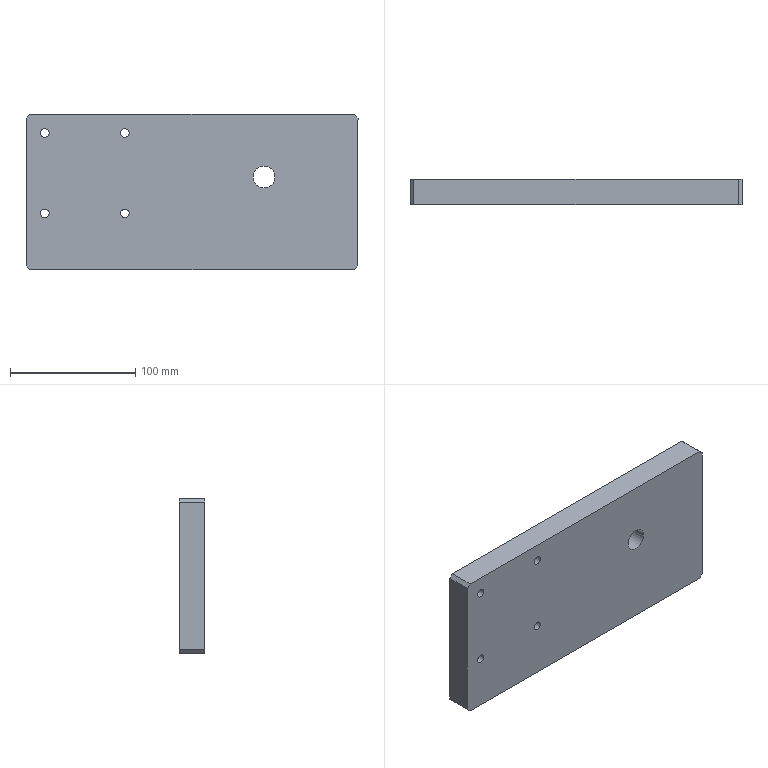Part | NX | 1 solid | 15 faces | box 265 x 20 x 124 mm | volume 649124 mm3 | plane 10 | cylinder 5 | commonest cylinder face diameters 6.8 x4 17.5 x1
STEP:
#1=CARTESIAN_POINT('',(-349.504,-20.,-263.815));
#2=VERTEX_POINT('',#1);
#3=CARTESIAN_POINT('',(-608.504,-20.,-263.815));
#4=VERTEX_POINT('',#3);
#5=CARTESIAN_POINT('',(-346.504,-20.,-263.815));
#6=DIRECTION('',(-1.,0.,0.));
#7=VECTOR('',#6,1000.);
#8=LINE('',#5,#7);
#9=EDGE_CURVE('',#2,#4,#8,.T.);
#10=ORIENTED_EDGE('',*,*,#9,.F.);
#11=CARTESIAN_POINT('',(-349.504,0.,-263.815));
#12=VERTEX_POINT('',#11);
#13=CARTESIAN_POINT('',(-349.504,-20.,-263.815));
#14=DIRECTION('',(0.,1.,0.));
#15=VECTOR('',#14,1000.);
#16=LINE('',#13,#15);
#17=EDGE_CURVE('',#2,#12,#16,.T.);
#18=ORIENTED_EDGE('',*,*,#17,.T.);
#19=CARTESIAN_POINT('',(-608.504,0.,-263.815));
#20=VERTEX_POINT('',#19);
#21=CARTESIAN_POINT('',(-346.504,0.,-263.815));
#22=DIRECTION('',(-1.,0.,0.));
#23=VECTOR('',#22,1000.);
#24=LINE('',#21,#23);
#25=EDGE_CURVE('',#12,#20,#24,.T.);
#26=ORIENTED_EDGE('',*,*,#25,.T.);
#27=CARTESIAN_POINT('',(-608.504,-20.,-263.815));
#28=DIRECTION('',(0.,-1.,0.));
#29=VECTOR('',#28,1000.);
#30=LINE('',#27,#29);
#31=EDGE_CURVE('',#20,#4,#30,.T.);
#32=ORIENTED_EDGE('',*,*,#31,.T.);
#33=EDGE_LOOP('',(#10,#18,#26,#32));
#34=FACE_BOUND('',#33,.T.);
#35=CARTESIAN_POINT('',(-346.504,-20.,-263.815));
#36=DIRECTION('',(0.,0.,-1.));
#37=DIRECTION('',(-1.,0.,0.));
#38=AXIS2_PLACEMENT_3D('',#35,#36,#37);
#39=PLANE('',#38);
#40=ADVANCED_FACE('',(#34),#39,.F.);
#41=CARTESIAN_POINT('',(-611.504,0.,-266.815));
#42=VERTEX_POINT('',#41);
#43=CARTESIAN_POINT('',(-611.504,0.,-384.815));
#44=VERTEX_POINT('',#43);
#45=CARTESIAN_POINT('',(-611.504,0.,-263.815));
#46=DIRECTION('',(0.,0.,-1.));
#47=VECTOR('',#46,1000.);
#48=LINE('',#45,#47);
#49=EDGE_CURVE('',#42,#44,#48,.T.);
#50=ORIENTED_EDGE('',*,*,#49,.T.);
#51=CARTESIAN_POINT('',(-611.504,-20.,-384.815));
#52=VERTEX_POINT('',#51);
#53=CARTESIAN_POINT('',(-611.504,-20.,-384.815));
#54=DIRECTION('',(0.,-1.,0.));
#55=VECTOR('',#54,1000.);
#56=LINE('',#53,#55);
#57=EDGE_CURVE('',#44,#52,#56,.T.);
#58=ORIENTED_EDGE('',*,*,#57,.T.);
#59=CARTESIAN_POINT('',(-611.504,-20.,-266.815));
#60=VERTEX_POINT('',#59);
#61=CARTESIAN_POINT('',(-611.504,-20.,-263.815));
#62=DIRECTION('',(0.,0.,-1.));
#63=VECTOR('',#62,1000.);
#64=LINE('',#61,#63);
#65=EDGE_CURVE('',#60,#52,#64,.T.);
#66=ORIENTED_EDGE('',*,*,#65,.F.);
#67=CARTESIAN_POINT('',(-611.504,-20.,-266.815));
#68=DIRECTION('',(0.,1.,0.));
#69=VECTOR('',#68,1000.);
#70=LINE('',#67,#69);
#71=EDGE_CURVE('',#60,#42,#70,.T.);
#72=ORIENTED_EDGE('',*,*,#71,.T.);
#73=EDGE_LOOP('',(#50,#58,#66,#72));
#74=FACE_BOUND('',#73,.T.);
#75=CARTESIAN_POINT('',(-611.504,-20.,-263.815));
#76=DIRECTION('',(1.,0.,0.));
#77=DIRECTION('',(0.,0.,-1.));
#78=AXIS2_PLACEMENT_3D('',#75,#76,#77);
#79=PLANE('',#78);
#80=ADVANCED_FACE('',(#74),#79,.F.);
#81=CARTESIAN_POINT('',(-608.504,0.,-387.815));
#82=VERTEX_POINT('',#81);
#83=CARTESIAN_POINT('',(-349.504,0.,-387.815));
#84=VERTEX_POINT('',#83);
#85=CARTESIAN_POINT('',(-611.504,0.,-387.815));
#86=DIRECTION('',(1.,0.,0.));
#87=VECTOR('',#86,1000.);
#88=LINE('',#85,#87);
#89=EDGE_CURVE('',#82,#84,#88,.T.);
#90=ORIENTED_EDGE('',*,*,#89,.T.);
#91=CARTESIAN_POINT('',(-349.504,-20.,-387.815));
#92=VERTEX_POINT('',#91);
#93=CARTESIAN_POINT('',(-349.504,-20.,-387.815));
#94=DIRECTION('',(0.,-1.,0.));
#95=VECTOR('',#94,1000.);
#96=LINE('',#93,#95);
#97=EDGE_CURVE('',#84,#92,#96,.T.);
#98=ORIENTED_EDGE('',*,*,#97,.T.);
#99=CARTESIAN_POINT('',(-608.504,-20.,-387.815));
#100=VERTEX_POINT('',#99);
#101=CARTESIAN_POINT('',(-611.504,-20.,-387.815));
#102=DIRECTION('',(1.,0.,0.));
#103=VECTOR('',#102,1000.);
#104=LINE('',#101,#103);
#105=EDGE_CURVE('',#100,#92,#104,.T.);
#106=ORIENTED_EDGE('',*,*,#105,.F.);
#107=CARTESIAN_POINT('',(-608.504,-20.,-387.815));
#108=DIRECTION('',(0.,1.,0.));
#109=VECTOR('',#108,1000.);
#110=LINE('',#107,#109);
#111=EDGE_CURVE('',#100,#82,#110,.T.);
#112=ORIENTED_EDGE('',*,*,#111,.T.);
#113=EDGE_LOOP('',(#90,#98,#106,#112));
#114=FACE_BOUND('',#113,.T.);
#115=CARTESIAN_POINT('',(-611.504,-20.,-387.815));
#116=DIRECTION('',(0.,0.,1.));
#117=DIRECTION('',(1.,0.,0.));
#118=AXIS2_PLACEMENT_3D('',#115,#116,#117);
#119=PLANE('',#118);
#120=ADVANCED_FACE('',(#114),#119,.F.);
#121=CARTESIAN_POINT('',(-346.504,0.,-384.815));
#122=VERTEX_POINT('',#121);
#123=CARTESIAN_POINT('',(-346.504,0.,-266.815));
#124=VERTEX_POINT('',#123);
#125=CARTESIAN_POINT('',(-346.504,0.,-387.815));
#126=DIRECTION('',(0.,0.,1.));
#127=VECTOR('',#126,1000.);
#128=LINE('',#125,#127);
#129=EDGE_CURVE('',#122,#124,#128,.T.);
#130=ORIENTED_EDGE('',*,*,#129,.T.);
#131=CARTESIAN_POINT('',(-346.504,-20.,-266.815));
#132=VERTEX_POINT('',#131);
#133=CARTESIAN_POINT('',(-346.504,-20.,-266.815));
#134=DIRECTION('',(0.,-1.,0.));
#135=VECTOR('',#134,1000.);
#136=LINE('',#133,#135);
#137=EDGE_CURVE('',#124,#132,#136,.T.);
#138=ORIENTED_EDGE('',*,*,#137,.T.);
#139=CARTESIAN_POINT('',(-346.504,-20.,-384.815));
#140=VERTEX_POINT('',#139);
#141=CARTESIAN_POINT('',(-346.504,-20.,-387.815));
#142=DIRECTION('',(0.,0.,1.));
#143=VECTOR('',#142,1000.);
#144=LINE('',#141,#143);
#145=EDGE_CURVE('',#140,#132,#144,.T.);
#146=ORIENTED_EDGE('',*,*,#145,.F.);
#147=CARTESIAN_POINT('',(-346.504,-20.,-384.815));
#148=DIRECTION('',(0.,1.,0.));
#149=VECTOR('',#148,1000.);
#150=LINE('',#147,#149);
#151=EDGE_CURVE('',#140,#122,#150,.T.);
#152=ORIENTED_EDGE('',*,*,#151,.T.);
#153=EDGE_LOOP('',(#130,#138,#146,#152));
#154=FACE_BOUND('',#153,.T.);
#155=CARTESIAN_POINT('',(-346.504,-20.,-387.815));
#156=DIRECTION('',(-1.,0.,0.));
#157=DIRECTION('',(0.,0.,1.));
#158=AXIS2_PLACEMENT_3D('',#155,#156,#157);
#159=PLANE('',#158);
#160=ADVANCED_FACE('',(#154),#159,.F.);
#161=CARTESIAN_POINT('',(-421.504,-20.,-322.565));
#162=VERTEX_POINT('',#161);
#163=CARTESIAN_POINT('',(-421.504,-20.,-313.815));
#164=DIRECTION('',(0.,-1.,0.));
#165=DIRECTION('',(0.,0.,-1.));
#166=AXIS2_PLACEMENT_3D('',#163,#164,#165);
#167=CIRCLE('',#166,8.75);
#168=EDGE_CURVE('',#162,#162,#167,.T.);
#169=ORIENTED_EDGE('',*,*,#168,.F.);
#170=EDGE_LOOP('',(#169));
#171=FACE_BOUND('',#170,.T.);
#172=CARTESIAN_POINT('',(-596.504,-20.,-346.215));
#173=VERTEX_POINT('',#172);
#174=CARTESIAN_POINT('',(-596.504,-20.,-342.815));
#175=DIRECTION('',(0.,-1.,0.));
#176=DIRECTION('',(0.,0.,-1.));
#177=AXIS2_PLACEMENT_3D('',#174,#175,#176);
#178=CIRCLE('',#177,3.4);
#179=EDGE_CURVE('',#173,#173,#178,.T.);
#180=ORIENTED_EDGE('',*,*,#179,.F.);
#181=EDGE_LOOP('',(#180));
#182=FACE_BOUND('',#181,.T.);
#183=CARTESIAN_POINT('',(-596.504,-20.,-282.215));
#184=VERTEX_POINT('',#183);
#185=CARTESIAN_POINT('',(-596.504,-20.,-278.815));
#186=DIRECTION('',(0.,-1.,0.));
#187=DIRECTION('',(0.,0.,-1.));
#188=AXIS2_PLACEMENT_3D('',#185,#186,#187);
#189=CIRCLE('',#188,3.4);
#190=EDGE_CURVE('',#184,#184,#189,.T.);
#191=ORIENTED_EDGE('',*,*,#190,.F.);
#192=EDGE_LOOP('',(#191));
#193=FACE_BOUND('',#192,.T.);
#194=CARTESIAN_POINT('',(-532.504,-20.,-346.215));
#195=VERTEX_POINT('',#194);
#196=CARTESIAN_POINT('',(-532.504,-20.,-342.815));
#197=DIRECTION('',(0.,-1.,0.));
#198=DIRECTION('',(0.,0.,-1.));
#199=AXIS2_PLACEMENT_3D('',#196,#197,#198);
#200=CIRCLE('',#199,3.4);
#201=EDGE_CURVE('',#195,#195,#200,.T.);
#202=ORIENTED_EDGE('',*,*,#201,.F.);
#203=EDGE_LOOP('',(#202));
#204=FACE_BOUND('',#203,.T.);
#205=CARTESIAN_POINT('',(-532.504,-20.,-282.215));
#206=VERTEX_POINT('',#205);
#207=CARTESIAN_POINT('',(-532.504,-20.,-278.815));
#208=DIRECTION('',(0.,-1.,0.));
#209=DIRECTION('',(0.,0.,-1.));
#210=AXIS2_PLACEMENT_3D('',#207,#208,#209);
#211=CIRCLE('',#210,3.4);
#212=EDGE_CURVE('',#206,#206,#211,.T.);
#213=ORIENTED_EDGE('',*,*,#212,.F.);
#214=EDGE_LOOP('',(#213));
#215=FACE_BOUND('',#214,.T.);
#216=ORIENTED_EDGE('',*,*,#145,.T.);
#217=CARTESIAN_POINT('',(-480.504,-20.,-132.815));
#218=DIRECTION('',(0.7071,0.,-0.7071));
#219=VECTOR('',#218,1000.);
#220=LINE('',#217,#219);
#221=EDGE_CURVE('',#132,#2,#220,.F.);
#222=ORIENTED_EDGE('',*,*,#221,.T.);
#223=ORIENTED_EDGE('',*,*,#9,.T.);
#224=CARTESIAN_POINT('',(-610.004,-20.,-265.315));
#225=DIRECTION('',(0.7071,0.,0.7071));
#226=VECTOR('',#225,1000.);
#227=LINE('',#224,#226);
#228=EDGE_CURVE('',#4,#60,#227,.F.);
#229=ORIENTED_EDGE('',*,*,#228,.T.);
#230=ORIENTED_EDGE('',*,*,#65,.T.);
#231=CARTESIAN_POINT('',(-672.004,-20.,-324.315));
#232=DIRECTION('',(-0.7071,0.,0.7071));
#233=VECTOR('',#232,1000.);
#234=LINE('',#231,#233);
#235=EDGE_CURVE('',#52,#100,#234,.F.);
#236=ORIENTED_EDGE('',*,*,#235,.T.);
#237=ORIENTED_EDGE('',*,*,#105,.T.);
#238=CARTESIAN_POINT('',(-418.504,-20.,-456.815));
#239=DIRECTION('',(-0.7071,0.,-0.7071));
#240=VECTOR('',#239,1000.);
#241=LINE('',#238,#240);
#242=EDGE_CURVE('',#92,#140,#241,.F.);
#243=ORIENTED_EDGE('',*,*,#242,.T.);
#244=EDGE_LOOP('',(#216,#222,#223,#229,#230,#236,#237,#243));
#245=FACE_BOUND('',#244,.T.);
#246=CARTESIAN_POINT('',(-611.504,-20.,-263.815));
#247=DIRECTION('',(0.,-1.,0.));
#248=DIRECTION('',(0.,0.,-1.));
#249=AXIS2_PLACEMENT_3D('',#246,#247,#248);
#250=PLANE('',#249);
#251=ADVANCED_FACE('',(#171,#182,#193,#204,#215,#245),#250,.T.);
#252=CARTESIAN_POINT('',(-421.504,0.,-322.565));
#253=VERTEX_POINT('',#252);
#254=CARTESIAN_POINT('',(-421.504,0.,-313.815));
#255=DIRECTION('',(0.,-1.,0.));
#256=DIRECTION('',(0.,0.,-1.));
#257=AXIS2_PLACEMENT_3D('',#254,#255,#256);
#258=CIRCLE('',#257,8.75);
#259=EDGE_CURVE('',#253,#253,#258,.T.);
#260=ORIENTED_EDGE('',*,*,#259,.T.);
#261=EDGE_LOOP('',(#260));
#262=FACE_BOUND('',#261,.T.);
#263=CARTESIAN_POINT('',(-596.504,0.,-346.215));
#264=VERTEX_POINT('',#263);
#265=CARTESIAN_POINT('',(-596.504,0.,-342.815));
#266=DIRECTION('',(0.,-1.,0.));
#267=DIRECTION('',(0.,0.,-1.));
#268=AXIS2_PLACEMENT_3D('',#265,#266,#267);
#269=CIRCLE('',#268,3.4);
#270=EDGE_CURVE('',#264,#264,#269,.T.);
#271=ORIENTED_EDGE('',*,*,#270,.T.);
#272=EDGE_LOOP('',(#271));
#273=FACE_BOUND('',#272,.T.);
#274=CARTESIAN_POINT('',(-596.504,0.,-282.215));
#275=VERTEX_POINT('',#274);
#276=CARTESIAN_POINT('',(-596.504,0.,-278.815));
#277=DIRECTION('',(0.,-1.,0.));
#278=DIRECTION('',(0.,0.,-1.));
#279=AXIS2_PLACEMENT_3D('',#276,#277,#278);
#280=CIRCLE('',#279,3.4);
#281=EDGE_CURVE('',#275,#275,#280,.T.);
#282=ORIENTED_EDGE('',*,*,#281,.T.);
#283=EDGE_LOOP('',(#282));
#284=FACE_BOUND('',#283,.T.);
#285=CARTESIAN_POINT('',(-532.504,0.,-346.215));
#286=VERTEX_POINT('',#285);
#287=CARTESIAN_POINT('',(-532.504,0.,-342.815));
#288=DIRECTION('',(0.,-1.,0.));
#289=DIRECTION('',(0.,0.,-1.));
#290=AXIS2_PLACEMENT_3D('',#287,#288,#289);
#291=CIRCLE('',#290,3.4);
#292=EDGE_CURVE('',#286,#286,#291,.T.);
#293=ORIENTED_EDGE('',*,*,#292,.T.);
#294=EDGE_LOOP('',(#293));
#295=FACE_BOUND('',#294,.T.);
#296=CARTESIAN_POINT('',(-532.504,0.,-282.215));
#297=VERTEX_POINT('',#296);
#298=CARTESIAN_POINT('',(-532.504,0.,-278.815));
#299=DIRECTION('',(0.,-1.,0.));
#300=DIRECTION('',(0.,0.,-1.));
#301=AXIS2_PLACEMENT_3D('',#298,#299,#300);
#302=CIRCLE('',#301,3.4);
#303=EDGE_CURVE('',#297,#297,#302,.T.);
#304=ORIENTED_EDGE('',*,*,#303,.T.);
#305=EDGE_LOOP('',(#304));
#306=FACE_BOUND('',#305,.T.);
#307=ORIENTED_EDGE('',*,*,#25,.F.);
#308=CARTESIAN_POINT('',(-349.504,0.,-263.815));
#309=DIRECTION('',(-0.7071,0.,0.7071));
#310=VECTOR('',#309,1000.);
#311=LINE('',#308,#310);
#312=EDGE_CURVE('',#12,#124,#311,.F.);
#313=ORIENTED_EDGE('',*,*,#312,.T.);
#314=ORIENTED_EDGE('',*,*,#129,.F.);
#315=CARTESIAN_POINT('',(-346.504,0.,-384.815));
#316=DIRECTION('',(0.7071,0.,0.7071));
#317=VECTOR('',#316,1000.);
#318=LINE('',#315,#317);
#319=EDGE_CURVE('',#122,#84,#318,.F.);
#320=ORIENTED_EDGE('',*,*,#319,.T.);
#321=ORIENTED_EDGE('',*,*,#89,.F.);
#322=CARTESIAN_POINT('',(-608.504,0.,-387.815));
#323=DIRECTION('',(0.7071,0.,-0.7071));
#324=VECTOR('',#323,1000.);
#325=LINE('',#322,#324);
#326=EDGE_CURVE('',#82,#44,#325,.F.);
#327=ORIENTED_EDGE('',*,*,#326,.T.);
#328=ORIENTED_EDGE('',*,*,#49,.F.);
#329=CARTESIAN_POINT('',(-611.504,0.,-266.815));
#330=DIRECTION('',(-0.7071,0.,-0.7071));
#331=VECTOR('',#330,1000.);
#332=LINE('',#329,#331);
#333=EDGE_CURVE('',#42,#20,#332,.F.);
#334=ORIENTED_EDGE('',*,*,#333,.T.);
#335=EDGE_LOOP('',(#307,#313,#314,#320,#321,#327,#328,#334));
#336=FACE_BOUND('',#335,.T.);
#337=CARTESIAN_POINT('',(-611.504,0.,-263.815));
#338=DIRECTION('',(0.,-1.,0.));
#339=DIRECTION('',(0.,0.,-1.));
#340=AXIS2_PLACEMENT_3D('',#337,#338,#339);
#341=PLANE('',#340);
#342=ADVANCED_FACE('',(#262,#273,#284,#295,#306,#336),#341,.F.);
#343=ORIENTED_EDGE('',*,*,#303,.F.);
#344=EDGE_LOOP('',(#343));
#345=FACE_BOUND('',#344,.T.);
#346=ORIENTED_EDGE('',*,*,#212,.T.);
#347=EDGE_LOOP('',(#346));
#348=FACE_BOUND('',#347,.T.);
#349=CARTESIAN_POINT('',(-532.504,-20.,-278.815));
#350=DIRECTION('',(0.,-1.,0.));
#351=DIRECTION('',(0.,0.,-1.));
#352=AXIS2_PLACEMENT_3D('',#349,#350,#351);
#353=CYLINDRICAL_SURFACE('',#352,3.4);
#354=ADVANCED_FACE('',(#345,#348),#353,.F.);
#355=ORIENTED_EDGE('',*,*,#292,.F.);
#356=EDGE_LOOP('',(#355));
#357=FACE_BOUND('',#356,.T.);
#358=ORIENTED_EDGE('',*,*,#201,.T.);
#359=EDGE_LOOP('',(#358));
#360=FACE_BOUND('',#359,.T.);
#361=CARTESIAN_POINT('',(-532.504,-20.,-342.815));
#362=DIRECTION('',(0.,-1.,0.));
#363=DIRECTION('',(0.,0.,-1.));
#364=AXIS2_PLACEMENT_3D('',#361,#362,#363);
#365=CYLINDRICAL_SURFACE('',#364,3.4);
#366=ADVANCED_FACE('',(#357,#360),#365,.F.);
#367=ORIENTED_EDGE('',*,*,#281,.F.);
#368=EDGE_LOOP('',(#367));
#369=FACE_BOUND('',#368,.T.);
#370=ORIENTED_EDGE('',*,*,#190,.T.);
#371=EDGE_LOOP('',(#370));
#372=FACE_BOUND('',#371,.T.);
#373=CARTESIAN_POINT('',(-596.504,-20.,-278.815));
#374=DIRECTION('',(0.,-1.,0.));
#375=DIRECTION('',(0.,0.,-1.));
#376=AXIS2_PLACEMENT_3D('',#373,#374,#375);
#377=CYLINDRICAL_SURFACE('',#376,3.4);
#378=ADVANCED_FACE('',(#369,#372),#377,.F.);
#379=ORIENTED_EDGE('',*,*,#270,.F.);
#380=EDGE_LOOP('',(#379));
#381=FACE_BOUND('',#380,.T.);
#382=ORIENTED_EDGE('',*,*,#179,.T.);
#383=EDGE_LOOP('',(#382));
#384=FACE_BOUND('',#383,.T.);
#385=CARTESIAN_POINT('',(-596.504,-20.,-342.815));
#386=DIRECTION('',(0.,-1.,0.));
#387=DIRECTION('',(0.,0.,-1.));
#388=AXIS2_PLACEMENT_3D('',#385,#386,#387);
#389=CYLINDRICAL_SURFACE('',#388,3.4);
#390=ADVANCED_FACE('',(#381,#384),#389,.F.);
#391=ORIENTED_EDGE('',*,*,#259,.F.);
#392=EDGE_LOOP('',(#391));
#393=FACE_BOUND('',#392,.T.);
#394=ORIENTED_EDGE('',*,*,#168,.T.);
#395=EDGE_LOOP('',(#394));
#396=FACE_BOUND('',#395,.T.);
#397=CARTESIAN_POINT('',(-421.504,-20.,-313.815));
#398=DIRECTION('',(0.,-1.,0.));
#399=DIRECTION('',(0.,0.,-1.));
#400=AXIS2_PLACEMENT_3D('',#397,#398,#399);
#401=CYLINDRICAL_SURFACE('',#400,8.75);
#402=ADVANCED_FACE('',(#393,#396),#401,.F.);
#403=ORIENTED_EDGE('',*,*,#221,.F.);
#404=ORIENTED_EDGE('',*,*,#137,.F.);
#405=ORIENTED_EDGE('',*,*,#312,.F.);
#406=ORIENTED_EDGE('',*,*,#17,.F.);
#407=EDGE_LOOP('',(#403,#404,#405,#406));
#408=FACE_BOUND('',#407,.T.);
#409=CARTESIAN_POINT('',(-349.504,-20.,-263.815));
#410=DIRECTION('',(-0.7071,0.,-0.7071));
#411=DIRECTION('',(0.,1.,0.));
#412=AXIS2_PLACEMENT_3D('',#409,#410,#411);
#413=PLANE('',#412);
#414=ADVANCED_FACE('',(#408),#413,.F.);
#415=ORIENTED_EDGE('',*,*,#242,.F.);
#416=ORIENTED_EDGE('',*,*,#97,.F.);
#417=ORIENTED_EDGE('',*,*,#319,.F.);
#418=ORIENTED_EDGE('',*,*,#151,.F.);
#419=EDGE_LOOP('',(#415,#416,#417,#418));
#420=FACE_BOUND('',#419,.T.);
#421=CARTESIAN_POINT('',(-346.504,-20.,-384.815));
#422=DIRECTION('',(-0.7071,0.,0.7071));
#423=DIRECTION('',(0.,1.,0.));
#424=AXIS2_PLACEMENT_3D('',#421,#422,#423);
#425=PLANE('',#424);
#426=ADVANCED_FACE('',(#420),#425,.F.);
#427=ORIENTED_EDGE('',*,*,#235,.F.);
#428=ORIENTED_EDGE('',*,*,#57,.F.);
#429=ORIENTED_EDGE('',*,*,#326,.F.);
#430=ORIENTED_EDGE('',*,*,#111,.F.);
#431=EDGE_LOOP('',(#427,#428,#429,#430));
#432=FACE_BOUND('',#431,.T.);
#433=CARTESIAN_POINT('',(-608.504,-20.,-387.815));
#434=DIRECTION('',(0.7071,0.,0.7071));
#435=DIRECTION('',(0.,1.,0.));
#436=AXIS2_PLACEMENT_3D('',#433,#434,#435);
#437=PLANE('',#436);
#438=ADVANCED_FACE('',(#432),#437,.F.);
#439=ORIENTED_EDGE('',*,*,#228,.F.);
#440=ORIENTED_EDGE('',*,*,#31,.F.);
#441=ORIENTED_EDGE('',*,*,#333,.F.);
#442=ORIENTED_EDGE('',*,*,#71,.F.);
#443=EDGE_LOOP('',(#439,#440,#441,#442));
#444=FACE_BOUND('',#443,.T.);
#445=CARTESIAN_POINT('',(-611.504,-20.,-266.815));
#446=DIRECTION('',(0.7071,0.,-0.7071));
#447=DIRECTION('',(0.,1.,0.));
#448=AXIS2_PLACEMENT_3D('',#445,#446,#447);
#449=PLANE('',#448);
#450=ADVANCED_FACE('',(#444),#449,.F.);
#451=CLOSED_SHELL('',(#40,#80,#120,#160,#251,#342,#354,#366,#378,#390,#402,#414,#426,#438,#450));
#452=MANIFOLD_SOLID_BREP('',#451);
#453=(LENGTH_UNIT()NAMED_UNIT(*)SI_UNIT(.MILLI.,.METRE.));
#454=UNCERTAINTY_MEASURE_WITH_UNIT(LENGTH_MEASURE(0.00001),#453,'','');
#455=(NAMED_UNIT(*)PLANE_ANGLE_UNIT()SI_UNIT($,.RADIAN.));
#456=(NAMED_UNIT(*)SI_UNIT($,.STERADIAN.)SOLID_ANGLE_UNIT());
#457=(GEOMETRIC_REPRESENTATION_CONTEXT(3)GLOBAL_UNCERTAINTY_ASSIGNED_CONTEXT((#454))GLOBAL_UNIT_ASSIGNED_CONTEXT((#453,#455,#456))REPRESENTATION_CONTEXT('',''));
#458=ADVANCED_BREP_SHAPE_REPRESENTATION('',(#452),#457);